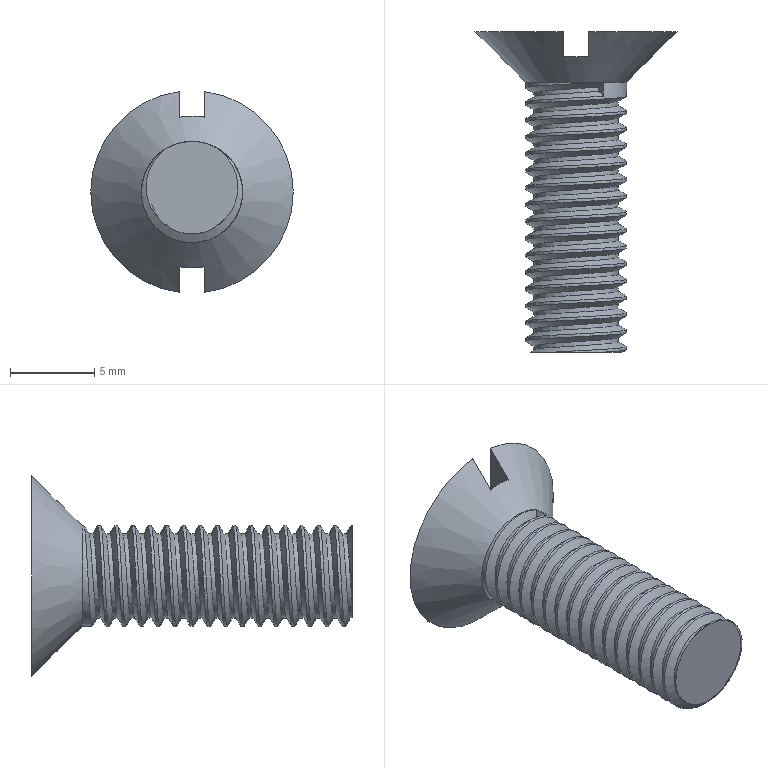Part | NX | features DATUM_CSYS 4, SKETCH 3, EXTRUDE 2, SWP104 1, THREADS 1 | 1 solid | 12 faces | box 12 x 19 x 11.906 mm | volume 533.089 mm3 | plane 7 | cylinder 2 | spline 2 | cone 1 | commonest cylinder face diameters 5 x1 6 x1